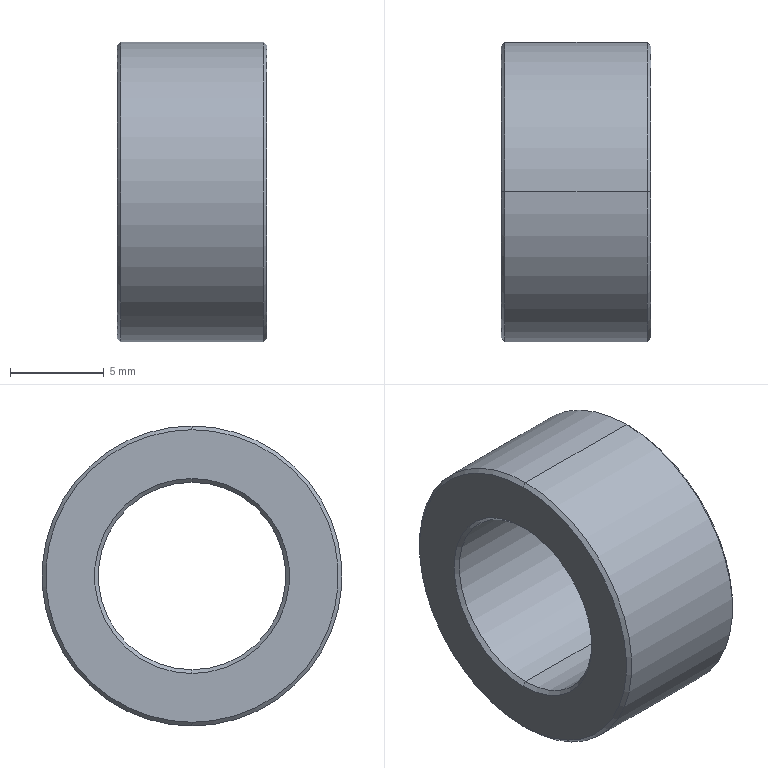Part | STEP file | WSSM16-10-8-23 | 1 solid | 14 faces | box 8 x 16 x 16 mm | volume 976.91 mm3 | cone 8 | cylinder 4 | plane 2 | commonest cylinder face diameters 10 x2 16 x2
STEP:
#1=CARTESIAN_POINT('',(8.,0.,-7.8));
#2=VERTEX_POINT('',#1);
#3=CARTESIAN_POINT('',(8.,0.,7.8));
#4=VERTEX_POINT('',#3);
#5=CARTESIAN_POINT('',(8.,0.,0.));
#6=DIRECTION('',(1.,0.,0.));
#7=DIRECTION('',(0.,0.,1.));
#8=AXIS2_PLACEMENT_3D('',#5,#6,#7);
#9=CIRCLE('',#8,7.8);
#10=EDGE_CURVE('',#2,#4,#9,.T.);
#11=ORIENTED_EDGE('',*,*,#10,.F.);
#12=CARTESIAN_POINT('',(7.8,0.,-8.));
#13=VERTEX_POINT('',#12);
#14=CARTESIAN_POINT('',(7.8,0.,-8.));
#15=DIRECTION('',(-0.7071,0.,-0.7071));
#16=VECTOR('',#15,1000.);
#17=LINE('',#14,#16);
#18=EDGE_CURVE('',#2,#13,#17,.T.);
#19=ORIENTED_EDGE('',*,*,#18,.T.);
#20=CARTESIAN_POINT('',(7.8,0.,8.));
#21=VERTEX_POINT('',#20);
#22=CARTESIAN_POINT('',(7.8,0.,0.));
#23=DIRECTION('',(-1.,0.,0.));
#24=DIRECTION('',(0.,0.,1.));
#25=AXIS2_PLACEMENT_3D('',#22,#23,#24);
#26=CIRCLE('',#25,8.);
#27=EDGE_CURVE('',#21,#13,#26,.T.);
#28=ORIENTED_EDGE('',*,*,#27,.F.);
#29=CARTESIAN_POINT('',(7.8,0.,8.));
#30=DIRECTION('',(-0.7071,0.,0.7071));
#31=VECTOR('',#30,1000.);
#32=LINE('',#29,#31);
#33=EDGE_CURVE('',#4,#21,#32,.T.);
#34=ORIENTED_EDGE('',*,*,#33,.F.);
#35=EDGE_LOOP('',(#11,#19,#28,#34));
#36=FACE_OUTER_BOUND('',#35,.T.);
#37=CARTESIAN_POINT('',(7.8,0.,0.));
#38=DIRECTION('',(-1.,0.,0.));
#39=DIRECTION('',(0.,0.,1.));
#40=AXIS2_PLACEMENT_3D('',#37,#38,#39);
#41=CONICAL_SURFACE('',#40,8.,0.7854);
#42=ADVANCED_FACE('',(#36),#41,.T.);
#43=CARTESIAN_POINT('',(7.8,0.,5.));
#44=VERTEX_POINT('',#43);
#45=CARTESIAN_POINT('',(7.8,0.,-5.));
#46=VERTEX_POINT('',#45);
#47=CARTESIAN_POINT('',(7.8,0.,0.));
#48=DIRECTION('',(1.,0.,0.));
#49=DIRECTION('',(0.,0.,1.));
#50=AXIS2_PLACEMENT_3D('',#47,#48,#49);
#51=CIRCLE('',#50,5.);
#52=EDGE_CURVE('',#44,#46,#51,.T.);
#53=ORIENTED_EDGE('',*,*,#52,.F.);
#54=CARTESIAN_POINT('',(8.,0.,5.2));
#55=VERTEX_POINT('',#54);
#56=CARTESIAN_POINT('',(8.,0.,5.2));
#57=DIRECTION('',(0.7071,0.,0.7071));
#58=VECTOR('',#57,1000.);
#59=LINE('',#56,#58);
#60=EDGE_CURVE('',#44,#55,#59,.T.);
#61=ORIENTED_EDGE('',*,*,#60,.T.);
#62=CARTESIAN_POINT('',(8.,0.,-5.2));
#63=VERTEX_POINT('',#62);
#64=CARTESIAN_POINT('',(8.,0.,0.));
#65=DIRECTION('',(-1.,0.,0.));
#66=DIRECTION('',(0.,0.,1.));
#67=AXIS2_PLACEMENT_3D('',#64,#65,#66);
#68=CIRCLE('',#67,5.2);
#69=EDGE_CURVE('',#63,#55,#68,.T.);
#70=ORIENTED_EDGE('',*,*,#69,.F.);
#71=CARTESIAN_POINT('',(8.,0.,-5.2));
#72=DIRECTION('',(0.7071,0.,-0.7071));
#73=VECTOR('',#72,1000.);
#74=LINE('',#71,#73);
#75=EDGE_CURVE('',#46,#63,#74,.T.);
#76=ORIENTED_EDGE('',*,*,#75,.F.);
#77=EDGE_LOOP('',(#53,#61,#70,#76));
#78=FACE_OUTER_BOUND('',#77,.T.);
#79=CARTESIAN_POINT('',(8.,0.,0.));
#80=DIRECTION('',(1.,0.,0.));
#81=DIRECTION('',(0.,0.,-1.));
#82=AXIS2_PLACEMENT_3D('',#79,#80,#81);
#83=CONICAL_SURFACE('',#82,5.2,0.7854);
#84=ADVANCED_FACE('',(#78),#83,.F.);
#85=CARTESIAN_POINT('',(0.,0.,7.8));
#86=VERTEX_POINT('',#85);
#87=CARTESIAN_POINT('',(0.,0.,-7.8));
#88=VERTEX_POINT('',#87);
#89=CARTESIAN_POINT('',(0.,0.,0.));
#90=DIRECTION('',(-1.,0.,0.));
#91=DIRECTION('',(0.,0.,-1.));
#92=AXIS2_PLACEMENT_3D('',#89,#90,#91);
#93=CIRCLE('',#92,7.8);
#94=EDGE_CURVE('',#86,#88,#93,.T.);
#95=ORIENTED_EDGE('',*,*,#94,.F.);
#96=CARTESIAN_POINT('',(0.2,0.,8.));
#97=VERTEX_POINT('',#96);
#98=CARTESIAN_POINT('',(0.,0.,7.8));
#99=DIRECTION('',(0.7071,0.,0.7071));
#100=VECTOR('',#99,1000.);
#101=LINE('',#98,#100);
#102=EDGE_CURVE('',#86,#97,#101,.T.);
#103=ORIENTED_EDGE('',*,*,#102,.T.);
#104=CARTESIAN_POINT('',(0.2,0.,-8.));
#105=VERTEX_POINT('',#104);
#106=CARTESIAN_POINT('',(0.2,0.,0.));
#107=DIRECTION('',(1.,0.,0.));
#108=DIRECTION('',(0.,0.,-1.));
#109=AXIS2_PLACEMENT_3D('',#106,#107,#108);
#110=CIRCLE('',#109,8.);
#111=EDGE_CURVE('',#105,#97,#110,.T.);
#112=ORIENTED_EDGE('',*,*,#111,.F.);
#113=CARTESIAN_POINT('',(0.,0.,-7.8));
#114=DIRECTION('',(0.7071,0.,-0.7071));
#115=VECTOR('',#114,1000.);
#116=LINE('',#113,#115);
#117=EDGE_CURVE('',#88,#105,#116,.T.);
#118=ORIENTED_EDGE('',*,*,#117,.F.);
#119=EDGE_LOOP('',(#95,#103,#112,#118));
#120=FACE_OUTER_BOUND('',#119,.T.);
#121=CARTESIAN_POINT('',(0.,0.,0.));
#122=DIRECTION('',(1.,0.,0.));
#123=DIRECTION('',(0.,0.,-1.));
#124=AXIS2_PLACEMENT_3D('',#121,#122,#123);
#125=CONICAL_SURFACE('',#124,7.8,0.7854);
#126=ADVANCED_FACE('',(#120),#125,.T.);
#127=CARTESIAN_POINT('',(0.2,0.,-5.));
#128=VERTEX_POINT('',#127);
#129=CARTESIAN_POINT('',(0.2,0.,5.));
#130=VERTEX_POINT('',#129);
#131=CARTESIAN_POINT('',(0.2,0.,0.));
#132=DIRECTION('',(-1.,0.,0.));
#133=DIRECTION('',(0.,0.,-1.));
#134=AXIS2_PLACEMENT_3D('',#131,#132,#133);
#135=CIRCLE('',#134,5.);
#136=EDGE_CURVE('',#128,#130,#135,.T.);
#137=ORIENTED_EDGE('',*,*,#136,.F.);
#138=CARTESIAN_POINT('',(0.,0.,-5.2));
#139=VERTEX_POINT('',#138);
#140=CARTESIAN_POINT('',(0.2,0.,-5.));
#141=DIRECTION('',(-0.7071,0.,-0.7071));
#142=VECTOR('',#141,1000.);
#143=LINE('',#140,#142);
#144=EDGE_CURVE('',#128,#139,#143,.T.);
#145=ORIENTED_EDGE('',*,*,#144,.T.);
#146=CARTESIAN_POINT('',(0.,0.,5.2));
#147=VERTEX_POINT('',#146);
#148=CARTESIAN_POINT('',(0.,0.,0.));
#149=DIRECTION('',(1.,0.,0.));
#150=DIRECTION('',(0.,0.,-1.));
#151=AXIS2_PLACEMENT_3D('',#148,#149,#150);
#152=CIRCLE('',#151,5.2);
#153=EDGE_CURVE('',#147,#139,#152,.T.);
#154=ORIENTED_EDGE('',*,*,#153,.F.);
#155=CARTESIAN_POINT('',(0.2,0.,5.));
#156=DIRECTION('',(-0.7071,0.,0.7071));
#157=VECTOR('',#156,1000.);
#158=LINE('',#155,#157);
#159=EDGE_CURVE('',#130,#147,#158,.T.);
#160=ORIENTED_EDGE('',*,*,#159,.F.);
#161=EDGE_LOOP('',(#137,#145,#154,#160));
#162=FACE_OUTER_BOUND('',#161,.T.);
#163=CARTESIAN_POINT('',(0.2,0.,0.));
#164=DIRECTION('',(-1.,0.,0.));
#165=DIRECTION('',(0.,0.,1.));
#166=AXIS2_PLACEMENT_3D('',#163,#164,#165);
#167=CONICAL_SURFACE('',#166,5.,0.7854);
#168=ADVANCED_FACE('',(#162),#167,.F.);
#169=ORIENTED_EDGE('',*,*,#52,.T.);
#170=CARTESIAN_POINT('',(0.,0.,-5.));
#171=DIRECTION('',(-1.,0.,0.));
#172=VECTOR('',#171,1000.);
#173=LINE('',#170,#172);
#174=EDGE_CURVE('',#46,#128,#173,.T.);
#175=ORIENTED_EDGE('',*,*,#174,.T.);
#176=ORIENTED_EDGE('',*,*,#136,.T.);
#177=CARTESIAN_POINT('',(0.,0.,5.));
#178=DIRECTION('',(-1.,0.,0.));
#179=VECTOR('',#178,1000.);
#180=LINE('',#177,#179);
#181=EDGE_CURVE('',#44,#130,#180,.T.);
#182=ORIENTED_EDGE('',*,*,#181,.F.);
#183=EDGE_LOOP('',(#169,#175,#176,#182));
#184=FACE_OUTER_BOUND('',#183,.T.);
#185=CARTESIAN_POINT('',(0.,0.,0.));
#186=DIRECTION('',(-1.,0.,0.));
#187=DIRECTION('',(0.,0.,1.));
#188=AXIS2_PLACEMENT_3D('',#185,#186,#187);
#189=CYLINDRICAL_SURFACE('',#188,5.);
#190=ADVANCED_FACE('',(#184),#189,.F.);
#191=ORIENTED_EDGE('',*,*,#27,.T.);
#192=CARTESIAN_POINT('',(0.,0.,-8.));
#193=DIRECTION('',(-1.,0.,0.));
#194=VECTOR('',#193,1000.);
#195=LINE('',#192,#194);
#196=EDGE_CURVE('',#13,#105,#195,.T.);
#197=ORIENTED_EDGE('',*,*,#196,.T.);
#198=ORIENTED_EDGE('',*,*,#111,.T.);
#199=CARTESIAN_POINT('',(0.,0.,8.));
#200=DIRECTION('',(-1.,0.,0.));
#201=VECTOR('',#200,1000.);
#202=LINE('',#199,#201);
#203=EDGE_CURVE('',#21,#97,#202,.T.);
#204=ORIENTED_EDGE('',*,*,#203,.F.);
#205=EDGE_LOOP('',(#191,#197,#198,#204));
#206=FACE_OUTER_BOUND('',#205,.T.);
#207=CARTESIAN_POINT('',(0.,0.,0.));
#208=DIRECTION('',(-1.,0.,0.));
#209=DIRECTION('',(0.,0.,1.));
#210=AXIS2_PLACEMENT_3D('',#207,#208,#209);
#211=CYLINDRICAL_SURFACE('',#210,8.);
#212=ADVANCED_FACE('',(#206),#211,.T.);
#213=ORIENTED_EDGE('',*,*,#153,.T.);
#214=CARTESIAN_POINT('',(0.,0.,0.));
#215=DIRECTION('',(1.,0.,0.));
#216=DIRECTION('',(0.,0.,-1.));
#217=AXIS2_PLACEMENT_3D('',#214,#215,#216);
#218=CIRCLE('',#217,5.2);
#219=EDGE_CURVE('',#139,#147,#218,.T.);
#220=ORIENTED_EDGE('',*,*,#219,.T.);
#221=EDGE_LOOP('',(#213,#220));
#222=FACE_BOUND('',#221,.T.);
#223=CARTESIAN_POINT('',(0.,0.,0.));
#224=DIRECTION('',(-1.,0.,0.));
#225=DIRECTION('',(0.,0.,-1.));
#226=AXIS2_PLACEMENT_3D('',#223,#224,#225);
#227=CIRCLE('',#226,7.8);
#228=EDGE_CURVE('',#88,#86,#227,.T.);
#229=ORIENTED_EDGE('',*,*,#228,.T.);
#230=ORIENTED_EDGE('',*,*,#94,.T.);
#231=EDGE_LOOP('',(#229,#230));
#232=FACE_OUTER_BOUND('',#231,.T.);
#233=CARTESIAN_POINT('',(0.,5.,0.));
#234=DIRECTION('',(1.,0.,0.));
#235=DIRECTION('',(0.,0.,-1.));
#236=AXIS2_PLACEMENT_3D('',#233,#234,#235);
#237=PLANE('',#236);
#238=ADVANCED_FACE('',(#222,#232),#237,.F.);
#239=ORIENTED_EDGE('',*,*,#196,.F.);
#240=CARTESIAN_POINT('',(7.8,0.,0.));
#241=DIRECTION('',(-1.,0.,0.));
#242=DIRECTION('',(0.,0.,1.));
#243=AXIS2_PLACEMENT_3D('',#240,#241,#242);
#244=CIRCLE('',#243,8.);
#245=EDGE_CURVE('',#13,#21,#244,.T.);
#246=ORIENTED_EDGE('',*,*,#245,.T.);
#247=ORIENTED_EDGE('',*,*,#203,.T.);
#248=CARTESIAN_POINT('',(0.2,0.,0.));
#249=DIRECTION('',(1.,0.,0.));
#250=DIRECTION('',(0.,0.,-1.));
#251=AXIS2_PLACEMENT_3D('',#248,#249,#250);
#252=CIRCLE('',#251,8.);
#253=EDGE_CURVE('',#97,#105,#252,.T.);
#254=ORIENTED_EDGE('',*,*,#253,.T.);
#255=EDGE_LOOP('',(#239,#246,#247,#254));
#256=FACE_OUTER_BOUND('',#255,.T.);
#257=CARTESIAN_POINT('',(0.,0.,0.));
#258=DIRECTION('',(-1.,0.,0.));
#259=DIRECTION('',(0.,0.,1.));
#260=AXIS2_PLACEMENT_3D('',#257,#258,#259);
#261=CYLINDRICAL_SURFACE('',#260,8.);
#262=ADVANCED_FACE('',(#256),#261,.T.);
#263=ORIENTED_EDGE('',*,*,#69,.T.);
#264=CARTESIAN_POINT('',(8.,0.,0.));
#265=DIRECTION('',(-1.,0.,0.));
#266=DIRECTION('',(0.,0.,1.));
#267=AXIS2_PLACEMENT_3D('',#264,#265,#266);
#268=CIRCLE('',#267,5.2);
#269=EDGE_CURVE('',#55,#63,#268,.T.);
#270=ORIENTED_EDGE('',*,*,#269,.T.);
#271=EDGE_LOOP('',(#263,#270));
#272=FACE_BOUND('',#271,.T.);
#273=CARTESIAN_POINT('',(8.,0.,0.));
#274=DIRECTION('',(1.,0.,0.));
#275=DIRECTION('',(0.,0.,1.));
#276=AXIS2_PLACEMENT_3D('',#273,#274,#275);
#277=CIRCLE('',#276,7.8);
#278=EDGE_CURVE('',#4,#2,#277,.T.);
#279=ORIENTED_EDGE('',*,*,#278,.T.);
#280=ORIENTED_EDGE('',*,*,#10,.T.);
#281=EDGE_LOOP('',(#279,#280));
#282=FACE_OUTER_BOUND('',#281,.T.);
#283=CARTESIAN_POINT('',(8.,5.,0.));
#284=DIRECTION('',(-1.,0.,0.));
#285=DIRECTION('',(0.,0.,1.));
#286=AXIS2_PLACEMENT_3D('',#283,#284,#285);
#287=PLANE('',#286);
#288=ADVANCED_FACE('',(#272,#282),#287,.F.);
#289=ORIENTED_EDGE('',*,*,#174,.F.);
#290=CARTESIAN_POINT('',(7.8,0.,0.));
#291=DIRECTION('',(1.,0.,0.));
#292=DIRECTION('',(0.,0.,1.));
#293=AXIS2_PLACEMENT_3D('',#290,#291,#292);
#294=CIRCLE('',#293,5.);
#295=EDGE_CURVE('',#46,#44,#294,.T.);
#296=ORIENTED_EDGE('',*,*,#295,.T.);
#297=ORIENTED_EDGE('',*,*,#181,.T.);
#298=CARTESIAN_POINT('',(0.2,0.,0.));
#299=DIRECTION('',(-1.,0.,0.));
#300=DIRECTION('',(0.,0.,-1.));
#301=AXIS2_PLACEMENT_3D('',#298,#299,#300);
#302=CIRCLE('',#301,5.);
#303=EDGE_CURVE('',#130,#128,#302,.T.);
#304=ORIENTED_EDGE('',*,*,#303,.T.);
#305=EDGE_LOOP('',(#289,#296,#297,#304));
#306=FACE_OUTER_BOUND('',#305,.T.);
#307=CARTESIAN_POINT('',(0.,0.,0.));
#308=DIRECTION('',(-1.,0.,0.));
#309=DIRECTION('',(0.,0.,1.));
#310=AXIS2_PLACEMENT_3D('',#307,#308,#309);
#311=CYLINDRICAL_SURFACE('',#310,5.);
#312=ADVANCED_FACE('',(#306),#311,.F.);
#313=ORIENTED_EDGE('',*,*,#144,.F.);
#314=ORIENTED_EDGE('',*,*,#303,.F.);
#315=ORIENTED_EDGE('',*,*,#159,.T.);
#316=ORIENTED_EDGE('',*,*,#219,.F.);
#317=EDGE_LOOP('',(#313,#314,#315,#316));
#318=FACE_OUTER_BOUND('',#317,.T.);
#319=CARTESIAN_POINT('',(0.2,0.,0.));
#320=DIRECTION('',(-1.,0.,0.));
#321=DIRECTION('',(0.,0.,1.));
#322=AXIS2_PLACEMENT_3D('',#319,#320,#321);
#323=CONICAL_SURFACE('',#322,5.,0.7854);
#324=ADVANCED_FACE('',(#318),#323,.F.);
#325=ORIENTED_EDGE('',*,*,#102,.F.);
#326=ORIENTED_EDGE('',*,*,#228,.F.);
#327=ORIENTED_EDGE('',*,*,#117,.T.);
#328=ORIENTED_EDGE('',*,*,#253,.F.);
#329=EDGE_LOOP('',(#325,#326,#327,#328));
#330=FACE_OUTER_BOUND('',#329,.T.);
#331=CARTESIAN_POINT('',(0.,0.,0.));
#332=DIRECTION('',(1.,0.,0.));
#333=DIRECTION('',(0.,0.,-1.));
#334=AXIS2_PLACEMENT_3D('',#331,#332,#333);
#335=CONICAL_SURFACE('',#334,7.8,0.7854);
#336=ADVANCED_FACE('',(#330),#335,.T.);
#337=ORIENTED_EDGE('',*,*,#60,.F.);
#338=ORIENTED_EDGE('',*,*,#295,.F.);
#339=ORIENTED_EDGE('',*,*,#75,.T.);
#340=ORIENTED_EDGE('',*,*,#269,.F.);
#341=EDGE_LOOP('',(#337,#338,#339,#340));
#342=FACE_OUTER_BOUND('',#341,.T.);
#343=CARTESIAN_POINT('',(8.,0.,0.));
#344=DIRECTION('',(1.,0.,0.));
#345=DIRECTION('',(0.,0.,-1.));
#346=AXIS2_PLACEMENT_3D('',#343,#344,#345);
#347=CONICAL_SURFACE('',#346,5.2,0.7854);
#348=ADVANCED_FACE('',(#342),#347,.F.);
#349=ORIENTED_EDGE('',*,*,#18,.F.);
#350=ORIENTED_EDGE('',*,*,#278,.F.);
#351=ORIENTED_EDGE('',*,*,#33,.T.);
#352=ORIENTED_EDGE('',*,*,#245,.F.);
#353=EDGE_LOOP('',(#349,#350,#351,#352));
#354=FACE_OUTER_BOUND('',#353,.T.);
#355=CARTESIAN_POINT('',(7.8,0.,0.));
#356=DIRECTION('',(-1.,0.,0.));
#357=DIRECTION('',(0.,0.,1.));
#358=AXIS2_PLACEMENT_3D('',#355,#356,#357);
#359=CONICAL_SURFACE('',#358,8.,0.7854);
#360=ADVANCED_FACE('',(#354),#359,.T.);
#361=CLOSED_SHELL('',(#42,#84,#126,#168,#190,#212,#238,#262,#288,#312,#324,#336,#348,#360));
#362=MANIFOLD_SOLID_BREP('',#361);
#363=CARTESIAN_POINT('',(0.,0.,0.));
#364=DIRECTION('',(0.,0.,1.));
#365=DIRECTION('',(1.,0.,0.));
#366=AXIS2_PLACEMENT_3D('',#363,#364,#365);
#367=(LENGTH_UNIT()NAMED_UNIT(*)SI_UNIT(.MILLI.,.METRE.));
#368=UNCERTAINTY_MEASURE_WITH_UNIT(LENGTH_MEASURE(0.00001),#367,'','');
#369=(NAMED_UNIT(*)PLANE_ANGLE_UNIT()SI_UNIT($,.RADIAN.));
#370=(NAMED_UNIT(*)SI_UNIT($,.STERADIAN.)SOLID_ANGLE_UNIT());
#371=(GEOMETRIC_REPRESENTATION_CONTEXT(3)GLOBAL_UNCERTAINTY_ASSIGNED_CONTEXT((#368))GLOBAL_UNIT_ASSIGNED_CONTEXT((#367,#369,#370))REPRESENTATION_CONTEXT('',''));
#372=ADVANCED_BREP_SHAPE_REPRESENTATION('',(#362,#366),#371);